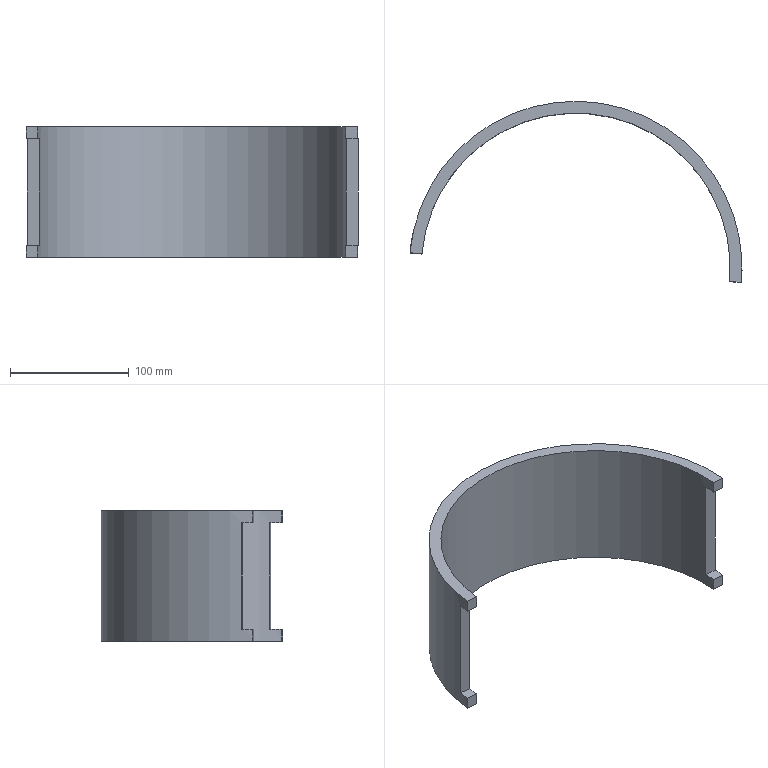Part | SolidWorks | features BaseBody 1 | 1 solid | 14 faces | box 279.443 x 152.477 x 110 mm | volume 448510 mm3 | plane 12 | cylinder 2 | commonest cylinder face diameters 260 x1 280 x1
STEP:
#1=CARTESIAN_POINT('',(399.859,1040.663,-284.893));
#2=VERTEX_POINT('',#1);
#3=CARTESIAN_POINT('',(399.859,1040.663,-294.893));
#4=VERTEX_POINT('',#3);
#5=CARTESIAN_POINT('',(399.859,1040.663,-184.893));
#6=DIRECTION('',(0.,0.,-1.));
#7=VECTOR('',#6,1000.);
#8=LINE('',#5,#7);
#9=EDGE_CURVE('',#2,#4,#8,.T.);
#10=ORIENTED_EDGE('',*,*,#9,.F.);
#11=CARTESIAN_POINT('',(389.899,1041.555,-284.893));
#12=VERTEX_POINT('',#11);
#13=CARTESIAN_POINT('',(946.393,991.761,-284.893));
#14=DIRECTION('',(-0.996,0.08912,0.));
#15=VECTOR('',#14,1000.);
#16=LINE('',#13,#15);
#17=EDGE_CURVE('',#2,#12,#16,.T.);
#18=ORIENTED_EDGE('',*,*,#17,.T.);
#19=CARTESIAN_POINT('',(389.899,1041.555,-294.893));
#20=VERTEX_POINT('',#19);
#21=CARTESIAN_POINT('',(389.899,1041.555,-184.893));
#22=DIRECTION('',(0.,0.,-1.));
#23=VECTOR('',#22,1000.);
#24=LINE('',#21,#23);
#25=EDGE_CURVE('',#12,#20,#24,.T.);
#26=ORIENTED_EDGE('',*,*,#25,.T.);
#27=CARTESIAN_POINT('',(260.416,1053.14,-294.893));
#28=DIRECTION('',(-0.996,0.08912,0.));
#29=VECTOR('',#28,1000.);
#30=LINE('',#27,#29);
#31=EDGE_CURVE('',#4,#20,#30,.T.);
#32=ORIENTED_EDGE('',*,*,#31,.F.);
#33=EDGE_LOOP('',(#10,#18,#26,#32));
#34=FACE_OUTER_BOUND('',#33,.T.);
#35=CARTESIAN_POINT('',(946.393,991.761,-284.893));
#36=DIRECTION('',(0.08912,0.996,0.));
#37=DIRECTION('',(0.,0.,-1.));
#38=AXIS2_PLACEMENT_3D('',#35,#36,#37);
#39=PLANE('',#38);
#40=ADVANCED_FACE('',(#34),#39,.F.);
#41=CARTESIAN_POINT('',(400.394,1050.655,-284.893));
#42=VERTEX_POINT('',#41);
#43=CARTESIAN_POINT('',(260.416,1053.14,-284.893));
#44=DIRECTION('',(0.,0.,-1.));
#45=DIRECTION('',(0.08912,0.996,0.));
#46=AXIS2_PLACEMENT_3D('',#43,#44,#45);
#47=CIRCLE('',#46,140.);
#48=EDGE_CURVE('',#42,#2,#47,.T.);
#49=ORIENTED_EDGE('',*,*,#48,.F.);
#50=CARTESIAN_POINT('',(390.406,1051.549,-284.893));
#51=VERTEX_POINT('',#50);
#52=CARTESIAN_POINT('',(947.285,1001.721,-284.893));
#53=DIRECTION('',(-0.996,0.08912,0.));
#54=VECTOR('',#53,1000.);
#55=LINE('',#52,#54);
#56=EDGE_CURVE('',#42,#51,#55,.T.);
#57=ORIENTED_EDGE('',*,*,#56,.T.);
#58=CARTESIAN_POINT('',(260.416,1053.14,-284.893));
#59=DIRECTION('',(0.,0.,-1.));
#60=DIRECTION('',(0.08912,0.996,0.));
#61=AXIS2_PLACEMENT_3D('',#58,#59,#60);
#62=CIRCLE('',#61,130.);
#63=EDGE_CURVE('',#51,#12,#62,.T.);
#64=ORIENTED_EDGE('',*,*,#63,.T.);
#65=ORIENTED_EDGE('',*,*,#17,.F.);
#66=EDGE_LOOP('',(#49,#57,#64,#65));
#67=FACE_OUTER_BOUND('',#66,.T.);
#68=CARTESIAN_POINT('',(946.393,991.761,-284.893));
#69=DIRECTION('',(0.,0.,-1.));
#70=DIRECTION('',(0.,-1.,0.));
#71=AXIS2_PLACEMENT_3D('',#68,#69,#70);
#72=PLANE('',#71);
#73=ADVANCED_FACE('',(#67),#72,.F.);
#74=CARTESIAN_POINT('',(400.394,1050.655,-194.893));
#75=VERTEX_POINT('',#74);
#76=CARTESIAN_POINT('',(400.394,1050.655,-184.893));
#77=DIRECTION('',(0.,0.,-1.));
#78=VECTOR('',#77,1000.);
#79=LINE('',#76,#78);
#80=EDGE_CURVE('',#75,#42,#79,.T.);
#81=ORIENTED_EDGE('',*,*,#80,.F.);
#82=CARTESIAN_POINT('',(390.406,1051.549,-194.893));
#83=VERTEX_POINT('',#82);
#84=CARTESIAN_POINT('',(947.285,1001.721,-194.893));
#85=DIRECTION('',(-0.996,0.08912,0.));
#86=VECTOR('',#85,1000.);
#87=LINE('',#84,#86);
#88=EDGE_CURVE('',#75,#83,#87,.T.);
#89=ORIENTED_EDGE('',*,*,#88,.T.);
#90=CARTESIAN_POINT('',(390.406,1051.549,-184.893));
#91=DIRECTION('',(0.,0.,-1.));
#92=VECTOR('',#91,1000.);
#93=LINE('',#90,#92);
#94=EDGE_CURVE('',#83,#51,#93,.T.);
#95=ORIENTED_EDGE('',*,*,#94,.T.);
#96=ORIENTED_EDGE('',*,*,#56,.F.);
#97=EDGE_LOOP('',(#81,#89,#95,#96));
#98=FACE_OUTER_BOUND('',#97,.T.);
#99=CARTESIAN_POINT('',(947.285,1001.721,-194.893));
#100=DIRECTION('',(0.08912,0.996,0.));
#101=DIRECTION('',(0.,0.,-1.));
#102=AXIS2_PLACEMENT_3D('',#99,#100,#101);
#103=PLANE('',#102);
#104=ADVANCED_FACE('',(#98),#103,.F.);
#105=CARTESIAN_POINT('',(399.859,1040.663,-194.893));
#106=VERTEX_POINT('',#105);
#107=CARTESIAN_POINT('',(260.416,1053.14,-194.893));
#108=DIRECTION('',(0.,0.,1.));
#109=DIRECTION('',(0.996,-0.08912,0.));
#110=AXIS2_PLACEMENT_3D('',#107,#108,#109);
#111=CIRCLE('',#110,140.);
#112=EDGE_CURVE('',#106,#75,#111,.T.);
#113=ORIENTED_EDGE('',*,*,#112,.F.);
#114=CARTESIAN_POINT('',(389.899,1041.555,-194.893));
#115=VERTEX_POINT('',#114);
#116=CARTESIAN_POINT('',(946.393,991.761,-194.893));
#117=DIRECTION('',(-0.996,0.08912,0.));
#118=VECTOR('',#117,1000.);
#119=LINE('',#116,#118);
#120=EDGE_CURVE('',#106,#115,#119,.T.);
#121=ORIENTED_EDGE('',*,*,#120,.T.);
#122=CARTESIAN_POINT('',(260.416,1053.14,-194.893));
#123=DIRECTION('',(0.,0.,1.));
#124=DIRECTION('',(0.996,-0.08912,0.));
#125=AXIS2_PLACEMENT_3D('',#122,#123,#124);
#126=CIRCLE('',#125,130.);
#127=EDGE_CURVE('',#115,#83,#126,.T.);
#128=ORIENTED_EDGE('',*,*,#127,.T.);
#129=ORIENTED_EDGE('',*,*,#88,.F.);
#130=EDGE_LOOP('',(#113,#121,#128,#129));
#131=FACE_OUTER_BOUND('',#130,.T.);
#132=CARTESIAN_POINT('',(947.285,1001.721,-194.893));
#133=DIRECTION('',(0.,0.,1.));
#134=DIRECTION('',(1.,0.,0.));
#135=AXIS2_PLACEMENT_3D('',#132,#133,#134);
#136=PLANE('',#135);
#137=ADVANCED_FACE('',(#131),#136,.F.);
#138=CARTESIAN_POINT('',(399.859,1040.663,-184.893));
#139=VERTEX_POINT('',#138);
#140=CARTESIAN_POINT('',(399.859,1040.663,-184.893));
#141=DIRECTION('',(0.,0.,-1.));
#142=VECTOR('',#141,1000.);
#143=LINE('',#140,#142);
#144=EDGE_CURVE('',#139,#106,#143,.T.);
#145=ORIENTED_EDGE('',*,*,#144,.F.);
#146=CARTESIAN_POINT('',(389.899,1041.555,-184.893));
#147=VERTEX_POINT('',#146);
#148=CARTESIAN_POINT('',(260.416,1053.14,-184.893));
#149=DIRECTION('',(-0.996,0.08912,0.));
#150=VECTOR('',#149,1000.);
#151=LINE('',#148,#150);
#152=EDGE_CURVE('',#139,#147,#151,.T.);
#153=ORIENTED_EDGE('',*,*,#152,.T.);
#154=CARTESIAN_POINT('',(389.899,1041.555,-184.893));
#155=DIRECTION('',(0.,0.,-1.));
#156=VECTOR('',#155,1000.);
#157=LINE('',#154,#156);
#158=EDGE_CURVE('',#147,#115,#157,.T.);
#159=ORIENTED_EDGE('',*,*,#158,.T.);
#160=ORIENTED_EDGE('',*,*,#120,.F.);
#161=EDGE_LOOP('',(#145,#153,#159,#160));
#162=FACE_OUTER_BOUND('',#161,.T.);
#163=CARTESIAN_POINT('',(946.393,991.761,-112.946));
#164=DIRECTION('',(0.08912,0.996,0.));
#165=DIRECTION('',(0.,0.,-1.));
#166=AXIS2_PLACEMENT_3D('',#163,#164,#165);
#167=PLANE('',#166);
#168=ADVANCED_FACE('',(#162),#167,.F.);
#169=CARTESIAN_POINT('',(120.973,1065.617,-194.893));
#170=VERTEX_POINT('',#169);
#171=CARTESIAN_POINT('',(120.973,1065.617,-184.893));
#172=VERTEX_POINT('',#171);
#173=CARTESIAN_POINT('',(120.973,1065.617,-184.893));
#174=DIRECTION('',(0.,0.,1.));
#175=VECTOR('',#174,1000.);
#176=LINE('',#173,#175);
#177=EDGE_CURVE('',#170,#172,#176,.T.);
#178=ORIENTED_EDGE('',*,*,#177,.F.);
#179=CARTESIAN_POINT('',(130.933,1064.726,-194.893));
#180=VERTEX_POINT('',#179);
#181=CARTESIAN_POINT('',(946.393,991.761,-194.893));
#182=DIRECTION('',(-0.996,0.08912,0.));
#183=VECTOR('',#182,1000.);
#184=LINE('',#181,#183);
#185=EDGE_CURVE('',#180,#170,#184,.T.);
#186=ORIENTED_EDGE('',*,*,#185,.F.);
#187=CARTESIAN_POINT('',(130.933,1064.726,-184.893));
#188=VERTEX_POINT('',#187);
#189=CARTESIAN_POINT('',(130.933,1064.726,-184.893));
#190=DIRECTION('',(0.,0.,1.));
#191=VECTOR('',#190,1000.);
#192=LINE('',#189,#191);
#193=EDGE_CURVE('',#180,#188,#192,.T.);
#194=ORIENTED_EDGE('',*,*,#193,.T.);
#195=CARTESIAN_POINT('',(260.416,1053.14,-184.893));
#196=DIRECTION('',(-0.996,0.08912,0.));
#197=VECTOR('',#196,1000.);
#198=LINE('',#195,#197);
#199=EDGE_CURVE('',#188,#172,#198,.T.);
#200=ORIENTED_EDGE('',*,*,#199,.T.);
#201=EDGE_LOOP('',(#178,#186,#194,#200));
#202=FACE_OUTER_BOUND('',#201,.T.);
#203=CARTESIAN_POINT('',(946.393,991.761,-112.946));
#204=DIRECTION('',(0.08912,0.996,0.));
#205=DIRECTION('',(0.,0.,-1.));
#206=AXIS2_PLACEMENT_3D('',#203,#204,#205);
#207=PLANE('',#206);
#208=ADVANCED_FACE('',(#202),#207,.F.);
#209=CARTESIAN_POINT('',(122.22,1075.546,-194.893));
#210=VERTEX_POINT('',#209);
#211=CARTESIAN_POINT('',(260.416,1053.14,-194.893));
#212=DIRECTION('',(0.,0.,1.));
#213=DIRECTION('',(0.996,-0.08912,0.));
#214=AXIS2_PLACEMENT_3D('',#211,#212,#213);
#215=CIRCLE('',#214,140.);
#216=EDGE_CURVE('',#210,#170,#215,.T.);
#217=ORIENTED_EDGE('',*,*,#216,.F.);
#218=CARTESIAN_POINT('',(132.208,1074.652,-194.893));
#219=VERTEX_POINT('',#218);
#220=CARTESIAN_POINT('',(947.285,1001.721,-194.893));
#221=DIRECTION('',(-0.996,0.08912,0.));
#222=VECTOR('',#221,1000.);
#223=LINE('',#220,#222);
#224=EDGE_CURVE('',#219,#210,#223,.T.);
#225=ORIENTED_EDGE('',*,*,#224,.F.);
#226=CARTESIAN_POINT('',(260.416,1053.14,-194.893));
#227=DIRECTION('',(0.,0.,1.));
#228=DIRECTION('',(0.996,-0.08912,0.));
#229=AXIS2_PLACEMENT_3D('',#226,#227,#228);
#230=CIRCLE('',#229,130.);
#231=EDGE_CURVE('',#219,#180,#230,.T.);
#232=ORIENTED_EDGE('',*,*,#231,.T.);
#233=ORIENTED_EDGE('',*,*,#185,.T.);
#234=EDGE_LOOP('',(#217,#225,#232,#233));
#235=FACE_OUTER_BOUND('',#234,.T.);
#236=CARTESIAN_POINT('',(947.285,1001.721,-194.893));
#237=DIRECTION('',(0.,0.,1.));
#238=DIRECTION('',(1.,0.,0.));
#239=AXIS2_PLACEMENT_3D('',#236,#237,#238);
#240=PLANE('',#239);
#241=ADVANCED_FACE('',(#235),#240,.F.);
#242=CARTESIAN_POINT('',(122.22,1075.546,-284.893));
#243=VERTEX_POINT('',#242);
#244=CARTESIAN_POINT('',(122.22,1075.546,-184.893));
#245=DIRECTION('',(0.,0.,1.));
#246=VECTOR('',#245,1000.);
#247=LINE('',#244,#246);
#248=EDGE_CURVE('',#243,#210,#247,.T.);
#249=ORIENTED_EDGE('',*,*,#248,.F.);
#250=CARTESIAN_POINT('',(132.208,1074.652,-284.893));
#251=VERTEX_POINT('',#250);
#252=CARTESIAN_POINT('',(947.285,1001.721,-284.893));
#253=DIRECTION('',(-0.996,0.08912,0.));
#254=VECTOR('',#253,1000.);
#255=LINE('',#252,#254);
#256=EDGE_CURVE('',#251,#243,#255,.T.);
#257=ORIENTED_EDGE('',*,*,#256,.F.);
#258=CARTESIAN_POINT('',(132.208,1074.652,-184.893));
#259=DIRECTION('',(0.,0.,1.));
#260=VECTOR('',#259,1000.);
#261=LINE('',#258,#260);
#262=EDGE_CURVE('',#251,#219,#261,.T.);
#263=ORIENTED_EDGE('',*,*,#262,.T.);
#264=ORIENTED_EDGE('',*,*,#224,.T.);
#265=EDGE_LOOP('',(#249,#257,#263,#264));
#266=FACE_OUTER_BOUND('',#265,.T.);
#267=CARTESIAN_POINT('',(947.285,1001.721,-194.893));
#268=DIRECTION('',(0.08912,0.996,0.));
#269=DIRECTION('',(0.,0.,-1.));
#270=AXIS2_PLACEMENT_3D('',#267,#268,#269);
#271=PLANE('',#270);
#272=ADVANCED_FACE('',(#266),#271,.F.);
#273=CARTESIAN_POINT('',(120.973,1065.617,-284.893));
#274=VERTEX_POINT('',#273);
#275=CARTESIAN_POINT('',(260.416,1053.14,-284.893));
#276=DIRECTION('',(0.,0.,-1.));
#277=DIRECTION('',(0.08912,0.996,0.));
#278=AXIS2_PLACEMENT_3D('',#275,#276,#277);
#279=CIRCLE('',#278,140.);
#280=EDGE_CURVE('',#274,#243,#279,.T.);
#281=ORIENTED_EDGE('',*,*,#280,.F.);
#282=CARTESIAN_POINT('',(130.933,1064.726,-284.893));
#283=VERTEX_POINT('',#282);
#284=CARTESIAN_POINT('',(946.393,991.761,-284.893));
#285=DIRECTION('',(-0.996,0.08912,0.));
#286=VECTOR('',#285,1000.);
#287=LINE('',#284,#286);
#288=EDGE_CURVE('',#283,#274,#287,.T.);
#289=ORIENTED_EDGE('',*,*,#288,.F.);
#290=CARTESIAN_POINT('',(260.416,1053.14,-284.893));
#291=DIRECTION('',(0.,0.,-1.));
#292=DIRECTION('',(0.08912,0.996,0.));
#293=AXIS2_PLACEMENT_3D('',#290,#291,#292);
#294=CIRCLE('',#293,130.);
#295=EDGE_CURVE('',#283,#251,#294,.T.);
#296=ORIENTED_EDGE('',*,*,#295,.T.);
#297=ORIENTED_EDGE('',*,*,#256,.T.);
#298=EDGE_LOOP('',(#281,#289,#296,#297));
#299=FACE_OUTER_BOUND('',#298,.T.);
#300=CARTESIAN_POINT('',(946.393,991.761,-284.893));
#301=DIRECTION('',(0.,0.,-1.));
#302=DIRECTION('',(0.,-1.,0.));
#303=AXIS2_PLACEMENT_3D('',#300,#301,#302);
#304=PLANE('',#303);
#305=ADVANCED_FACE('',(#299),#304,.F.);
#306=CARTESIAN_POINT('',(120.973,1065.617,-294.893));
#307=VERTEX_POINT('',#306);
#308=CARTESIAN_POINT('',(120.973,1065.617,-184.893));
#309=DIRECTION('',(0.,0.,1.));
#310=VECTOR('',#309,1000.);
#311=LINE('',#308,#310);
#312=EDGE_CURVE('',#307,#274,#311,.T.);
#313=ORIENTED_EDGE('',*,*,#312,.F.);
#314=CARTESIAN_POINT('',(130.933,1064.726,-294.893));
#315=VERTEX_POINT('',#314);
#316=CARTESIAN_POINT('',(260.416,1053.14,-294.893));
#317=DIRECTION('',(-0.996,0.08912,0.));
#318=VECTOR('',#317,1000.);
#319=LINE('',#316,#318);
#320=EDGE_CURVE('',#315,#307,#319,.T.);
#321=ORIENTED_EDGE('',*,*,#320,.F.);
#322=CARTESIAN_POINT('',(130.933,1064.726,-184.893));
#323=DIRECTION('',(0.,0.,1.));
#324=VECTOR('',#323,1000.);
#325=LINE('',#322,#324);
#326=EDGE_CURVE('',#315,#283,#325,.T.);
#327=ORIENTED_EDGE('',*,*,#326,.T.);
#328=ORIENTED_EDGE('',*,*,#288,.T.);
#329=EDGE_LOOP('',(#313,#321,#327,#328));
#330=FACE_OUTER_BOUND('',#329,.T.);
#331=CARTESIAN_POINT('',(946.393,991.761,-284.893));
#332=DIRECTION('',(0.08912,0.996,0.));
#333=DIRECTION('',(0.,0.,-1.));
#334=AXIS2_PLACEMENT_3D('',#331,#332,#333);
#335=PLANE('',#334);
#336=ADVANCED_FACE('',(#330),#335,.F.);
#337=ORIENTED_EDGE('',*,*,#158,.F.);
#338=CARTESIAN_POINT('',(260.416,1053.14,-184.893));
#339=DIRECTION('',(0.,0.,1.));
#340=DIRECTION('',(0.996,-0.08912,0.));
#341=AXIS2_PLACEMENT_3D('',#338,#339,#340);
#342=CIRCLE('',#341,130.);
#343=EDGE_CURVE('',#147,#188,#342,.T.);
#344=ORIENTED_EDGE('',*,*,#343,.T.);
#345=ORIENTED_EDGE('',*,*,#193,.F.);
#346=ORIENTED_EDGE('',*,*,#231,.F.);
#347=ORIENTED_EDGE('',*,*,#262,.F.);
#348=ORIENTED_EDGE('',*,*,#295,.F.);
#349=ORIENTED_EDGE('',*,*,#326,.F.);
#350=CARTESIAN_POINT('',(260.416,1053.14,-294.893));
#351=DIRECTION('',(0.,0.,1.));
#352=DIRECTION('',(0.996,-0.08912,0.));
#353=AXIS2_PLACEMENT_3D('',#350,#351,#352);
#354=CIRCLE('',#353,130.);
#355=EDGE_CURVE('',#20,#315,#354,.T.);
#356=ORIENTED_EDGE('',*,*,#355,.F.);
#357=ORIENTED_EDGE('',*,*,#25,.F.);
#358=ORIENTED_EDGE('',*,*,#63,.F.);
#359=ORIENTED_EDGE('',*,*,#94,.F.);
#360=ORIENTED_EDGE('',*,*,#127,.F.);
#361=EDGE_LOOP('',(#337,#344,#345,#346,#347,#348,#349,#356,#357,#358,#359,#360));
#362=FACE_OUTER_BOUND('',#361,.T.);
#363=CARTESIAN_POINT('',(260.416,1053.14,-184.893));
#364=DIRECTION('',(0.,0.,-1.));
#365=DIRECTION('',(0.996,-0.08912,0.));
#366=AXIS2_PLACEMENT_3D('',#363,#364,#365);
#367=CYLINDRICAL_SURFACE('',#366,130.);
#368=ADVANCED_FACE('',(#362),#367,.F.);
#369=CARTESIAN_POINT('',(260.416,1053.14,-184.893));
#370=DIRECTION('',(0.,0.,1.));
#371=DIRECTION('',(0.996,-0.08912,0.));
#372=AXIS2_PLACEMENT_3D('',#369,#370,#371);
#373=CIRCLE('',#372,140.);
#374=EDGE_CURVE('',#139,#172,#373,.T.);
#375=ORIENTED_EDGE('',*,*,#374,.F.);
#376=ORIENTED_EDGE('',*,*,#144,.T.);
#377=ORIENTED_EDGE('',*,*,#112,.T.);
#378=ORIENTED_EDGE('',*,*,#80,.T.);
#379=ORIENTED_EDGE('',*,*,#48,.T.);
#380=ORIENTED_EDGE('',*,*,#9,.T.);
#381=CARTESIAN_POINT('',(260.416,1053.14,-294.893));
#382=DIRECTION('',(0.,0.,1.));
#383=DIRECTION('',(0.996,-0.08912,0.));
#384=AXIS2_PLACEMENT_3D('',#381,#382,#383);
#385=CIRCLE('',#384,140.);
#386=EDGE_CURVE('',#4,#307,#385,.T.);
#387=ORIENTED_EDGE('',*,*,#386,.T.);
#388=ORIENTED_EDGE('',*,*,#312,.T.);
#389=ORIENTED_EDGE('',*,*,#280,.T.);
#390=ORIENTED_EDGE('',*,*,#248,.T.);
#391=ORIENTED_EDGE('',*,*,#216,.T.);
#392=ORIENTED_EDGE('',*,*,#177,.T.);
#393=EDGE_LOOP('',(#375,#376,#377,#378,#379,#380,#387,#388,#389,#390,#391,#392));
#394=FACE_OUTER_BOUND('',#393,.T.);
#395=CARTESIAN_POINT('',(260.416,1053.14,-184.893));
#396=DIRECTION('',(0.,0.,-1.));
#397=DIRECTION('',(0.996,-0.08912,0.));
#398=AXIS2_PLACEMENT_3D('',#395,#396,#397);
#399=CYLINDRICAL_SURFACE('',#398,140.);
#400=ADVANCED_FACE('',(#394),#399,.T.);
#401=ORIENTED_EDGE('',*,*,#386,.F.);
#402=ORIENTED_EDGE('',*,*,#31,.T.);
#403=ORIENTED_EDGE('',*,*,#355,.T.);
#404=ORIENTED_EDGE('',*,*,#320,.T.);
#405=EDGE_LOOP('',(#401,#402,#403,#404));
#406=FACE_OUTER_BOUND('',#405,.T.);
#407=CARTESIAN_POINT('',(260.416,1053.14,-294.893));
#408=DIRECTION('',(0.,0.,1.));
#409=DIRECTION('',(1.,0.,0.));
#410=AXIS2_PLACEMENT_3D('',#407,#408,#409);
#411=PLANE('',#410);
#412=ADVANCED_FACE('',(#406),#411,.F.);
#413=ORIENTED_EDGE('',*,*,#152,.F.);
#414=ORIENTED_EDGE('',*,*,#374,.T.);
#415=ORIENTED_EDGE('',*,*,#199,.F.);
#416=ORIENTED_EDGE('',*,*,#343,.F.);
#417=EDGE_LOOP('',(#413,#414,#415,#416));
#418=FACE_OUTER_BOUND('',#417,.T.);
#419=CARTESIAN_POINT('',(260.416,1053.14,-184.893));
#420=DIRECTION('',(0.,0.,1.));
#421=DIRECTION('',(1.,0.,0.));
#422=AXIS2_PLACEMENT_3D('',#419,#420,#421);
#423=PLANE('',#422);
#424=ADVANCED_FACE('',(#418),#423,.T.);
#425=CLOSED_SHELL('',(#40,#73,#104,#137,#168,#208,#241,#272,#305,#336,#368,#400,#412,#424));
#426=MANIFOLD_SOLID_BREP('',#425);
#427=CARTESIAN_POINT('',(0.,0.,0.));
#428=DIRECTION('',(0.,0.,1.));
#429=DIRECTION('',(1.,0.,0.));
#430=AXIS2_PLACEMENT_3D('',#427,#428,#429);
#431=(LENGTH_UNIT()NAMED_UNIT(*)SI_UNIT(.MILLI.,.METRE.));
#432=UNCERTAINTY_MEASURE_WITH_UNIT(LENGTH_MEASURE(0.00001),#431,'','');
#433=(NAMED_UNIT(*)PLANE_ANGLE_UNIT()SI_UNIT($,.RADIAN.));
#434=(NAMED_UNIT(*)SI_UNIT($,.STERADIAN.)SOLID_ANGLE_UNIT());
#435=(GEOMETRIC_REPRESENTATION_CONTEXT(3)GLOBAL_UNCERTAINTY_ASSIGNED_CONTEXT((#432))GLOBAL_UNIT_ASSIGNED_CONTEXT((#431,#433,#434))REPRESENTATION_CONTEXT('',''));
#436=ADVANCED_BREP_SHAPE_REPRESENTATION('',(#426,#430),#435);